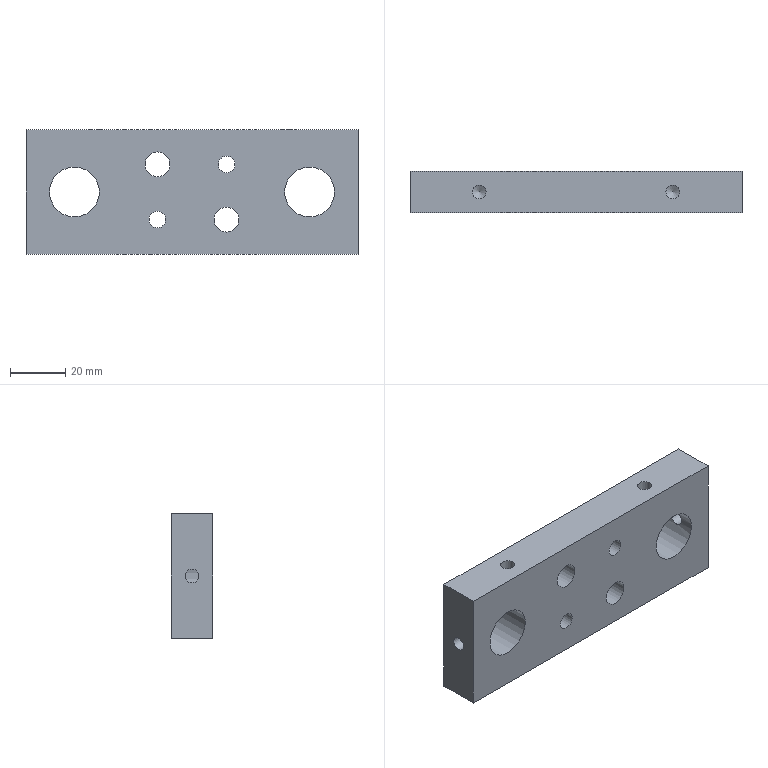Part | NX | features BREP 1 | 1 solid | 22 faces | box 120 x 15 x 45 mm | volume 67717 mm3 | cylinder 12 | plane 8 | cone 2 | commonest cylinder face diameters 5 x4 6 x2 9 x2 15 x2 18 x2